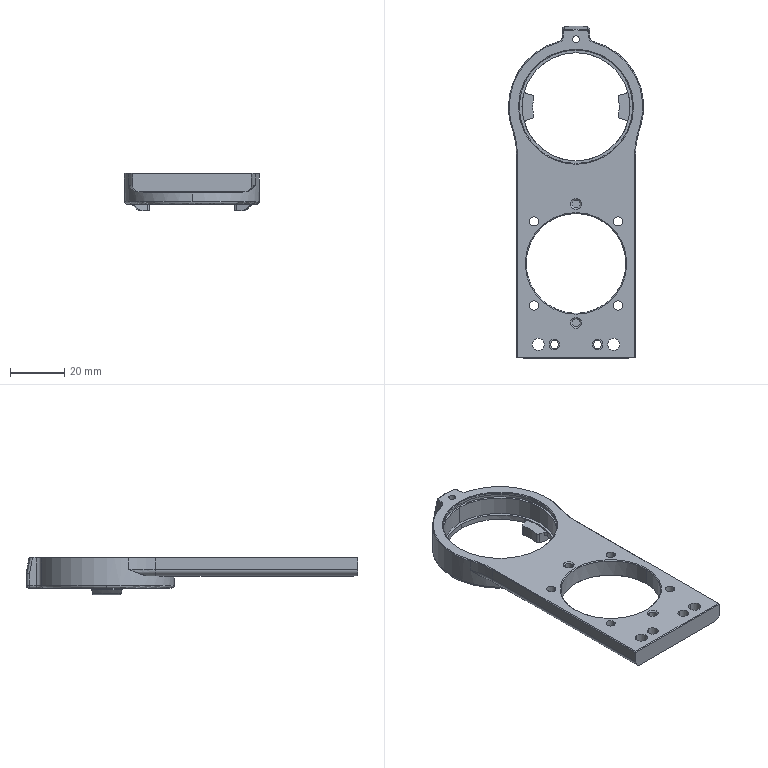NC program | NX | posted with a generic post | part box 50 x 122.9 x 14 mm
Lines 19 to 852 of 4462:
(ZLEVEL_PROFILE , TOOL : D10)
N36 T15 M6
N38 G54
N40 G17 G0 G90 X-66.55 Y-13.852 S9500 M3
N42 G43 Z30. H15
N44 Z1.5
N46 G94 G1 Y22.554 Z-0.408 F1000.
N48 X-66.216 Y23.898 Z-0.481
N50 X-65.534 Y25.104 Z-0.553
N52 X-64.554 Y26.084 Z-0.626
N54 X-63.348 Y26.766 Z-0.698
N56 X-62.004 Y27.1 Z-0.771
N58 X-61.45 Z-0.8
N60 X13.634 F3500.
N62 G3 X21.745 Y28.458 R24.9
N64 G2 X59.92 Y10.056 R30.1
N66 X65.193 Y4.632 R6.157
N68 X65.162 Y-4.852 R34.086
N70 X59.926 Y-10.04 R6.113
N72 X21.745 Y-28.458 R30.1
N74 G3 X13.634 Y-27.1 R24.9
N76 G1 X-61.45
N78 G2 X-66.55 Y-22. R5.1
N80 G1 Y22.
N82 G2 X-61.45 Y27.1 R5.1
N84 G1 X13.634 Z-0.973
N86 X14.666 Y27.121 Z-0.976
N88 X15.697 Y27.186 Z-0.978
N90 X16.724 Y27.293 Z-0.981
N92 X17.746 Y27.442 Z-0.983
N94 X18.76 Y27.634 Z-0.985
N96 X19.766 Y27.867 Z-0.988
N98 X20.762 Y28.142 Z-0.99
N100 X21.745 Y28.458 Z-0.992
N102 X22.988 Y28.857 Z-0.996
N104 X24.248 Y29.201 Z-0.999
N106 X25.522 Y29.49 Z-1.002
N108 X26.806 Y29.724 Z-1.005
N110 X28.1 Y29.902 Z-1.008
N112 X29.4 Y30.023 Z-1.011
N114 X30.704 Y30.088 Z-1.014
N116 X32.01 Y30.096 Z-1.017
N118 X33.315 Y30.048 Z-1.02
N120 X34.617 Y29.943 Z-1.023
N122 X35.913 Y29.782 Z-1.026
N124 X37.2 Y29.565 Z-1.029
N126 X38.478 Y29.292 Z-1.032
N128 X39.742 Y28.964 Z-1.035
N130 X40.99 Y28.581 Z-1.038
N132 X42.221 Y28.145 Z-1.041
N134 X43.432 Y27.656 Z-1.044
N136 X44.62 Y27.114 Z-1.047
N138 X45.784 Y26.522 Z-1.05
N140 X46.921 Y25.88 Z-1.053
N142 X48.029 Y25.188 Z-1.056
N144 X49.106 Y24.45 Z-1.059
N146 X50.15 Y23.666 Z-1.062
N148 X51.159 Y22.837 Z-1.065
N150 X52.131 Y21.965 Z-1.068
N152 X53.064 Y21.051 Z-1.071
N154 X53.957 Y20.098 Z-1.074
N156 X54.808 Y19.107 Z-1.077
N158 X55.615 Y18.081 Z-1.08
N160 X56.376 Y17.02 Z-1.083
N162 X57.091 Y15.927 Z-1.086
N164 X57.758 Y14.804 Z-1.089
N166 X58.375 Y13.654 Z-1.092
N168 X58.942 Y12.477 Z-1.095
N170 X59.452 Y11.291 Z-1.098
N172 X59.923 Y10.052 Z-1.101
N174 X60.494 Y9.952 Z-1.102
N176 X61.054 Y9.797 Z-1.104
N178 X61.6 Y9.593 Z-1.105
N180 X62.124 Y9.337 Z-1.106
N182 X62.376 Y9.189 Z-1.107
N184 X62.622 Y9.031 Z-1.108
N186 X62.859 Y8.861
N188 X63.085 Y8.674 Z-1.109
N190 X63.519 Y8.28 Z-1.11
N192 X63.913 Y7.846 Z-1.112
N194 X64.261 Y7.374 Z-1.113
N196 X64.566 Y6.872 Z-1.115
N198 X64.816 Y6.341 Z-1.116
N200 X65.015 Y5.787 Z-1.117
N202 X65.141 Y5.317 Z-1.118
N204 X65.23 Y4.838 Z-1.119
N206 X65.256 Y4.64 Z-1.12
N208 X65.393 Y3.457 Z-1.123
N210 X65.499 Y2.27 Z-1.125
N212 X65.558 Y1.08 Z-1.128
N214 X65.577 Y-0.111 Z-1.131
N216 X65.549 Y-1.303 Z-1.134
N218 X65.486 Y-2.492 Z-1.136
N220 X65.373 Y-3.679 Z-1.139
N222 X65.231 Y-4.862 Z-1.142
N224 X65.121 Y-5.423 Z-1.143
N226 X64.961 Y-5.971 Z-1.145
N228 X64.752 Y-6.503 Z-1.146
N230 X64.494 Y-7.012 Z-1.147
N232 X64.188 Y-7.493 Z-1.149
N234 X63.839 Y-7.945 Z-1.15
N236 X63.448 Y-8.36 Z-1.151
N238 X63.025 Y-8.74 Z-1.152
N240 X62.563 Y-9.073 Z-1.154
N242 X62.076 Y-9.366 Z-1.155
N244 X61.565 Y-9.614 Z-1.156
N246 X61.032 Y-9.807 Z-1.158
N248 X60.485 Y-9.957 Z-1.159
N250 X59.927 Y-10.05 Z-1.16
N252 X59.456 Y-11.281 Z-1.163
N254 X58.949 Y-12.463 Z-1.166
N256 X58.382 Y-13.64 Z-1.169
N258 X57.765 Y-14.791 Z-1.172
N260 X57.099 Y-15.915 Z-1.175
N262 X56.384 Y-17.008 Z-1.178
N264 X55.623 Y-18.07 Z-1.181
N266 X54.816 Y-19.097 Z-1.184
N268 X53.965 Y-20.089 Z-1.187
N270 X53.073 Y-21.042 Z-1.191
N272 X52.139 Y-21.956 Z-1.194
N274 X51.167 Y-22.829 Z-1.197
N276 X50.158 Y-23.659 Z-1.2
N278 X49.114 Y-24.444 Z-1.203
N280 X48.037 Y-25.183 Z-1.206
N282 X46.929 Y-25.875 Z-1.209
N284 X45.792 Y-26.518 Z-1.212
N286 X44.628 Y-27.111 Z-1.215
N288 X43.439 Y-27.653 Z-1.218
N290 X42.228 Y-28.142 Z-1.221
N292 X40.997 Y-28.579 Z-1.224
N294 X39.748 Y-28.962 Z-1.227
N296 X38.483 Y-29.291 Z-1.23
N298 X37.206 Y-29.564 Z-1.233
N300 X35.918 Y-29.781 Z-1.236
N302 X34.622 Y-29.943 Z-1.239
N304 X33.32 Y-30.048 Z-1.242
N306 X32.014 Y-30.096 Z-1.245
N308 X30.708 Y-30.088 Z-1.248
N310 X29.403 Y-30.023 Z-1.251
N312 X28.102 Y-29.902 Z-1.254
N314 X26.808 Y-29.724 Z-1.257
N316 X25.523 Y-29.49 Z-1.26
N318 X24.249 Y-29.201 Z-1.263
N320 X22.989 Y-28.857 Z-1.266
N322 X21.745 Y-28.458 Z-1.269
N324 X20.762 Y-28.142 Z-1.271
N326 X19.766 Y-27.867 Z-1.274
N328 X18.76 Y-27.634 Z-1.276
N330 X17.746 Y-27.442 Z-1.278
N332 X16.724 Y-27.293 Z-1.281
N334 X15.697 Y-27.186 Z-1.283
N336 X14.666 Y-27.121 Z-1.286
N338 X13.634 Y-27.1 Z-1.288
N340 X-61.45 Z-1.461
N342 X-61.95 Y-27.075 Z-1.463
N344 X-62.445 Y-27.002 Z-1.464
N346 X-62.93 Y-26.88 Z-1.465
N348 X-63.402 Y-26.712 Z-1.466
N350 X-63.854 Y-26.498 Z-1.467
N352 X-64.283 Y-26.24 Z-1.468
N354 X-64.685 Y-25.942 Z-1.47
N356 X-65.056 Y-25.606 Z-1.471
N358 X-65.392 Y-25.235 Z-1.472
N360 X-65.69 Y-24.833 Z-1.473
N362 X-65.948 Y-24.404 Z-1.474
N364 X-66.162 Y-23.952 Z-1.475
N366 X-66.33 Y-23.48 Z-1.476
N368 X-66.452 Y-22.995 Z-1.478
N370 X-66.525 Y-22.5 Z-1.479
N372 X-66.55 Y-22. Z-1.48
N374 Y22. Z-1.582
N376 X-66.525 Y22.5 Z-1.583
N378 X-66.452 Y22.995 Z-1.584
N380 X-66.33 Y23.48 Z-1.585
N382 X-66.162 Y23.952 Z-1.586
N384 X-65.948 Y24.404 Z-1.587
N386 X-65.69 Y24.833 Z-1.588
N388 X-65.392 Y25.235 Z-1.59
N390 X-65.056 Y25.606 Z-1.591
N392 X-64.685 Y25.942 Z-1.592
N394 X-64.283 Y26.24 Z-1.593
N396 X-63.854 Y26.498 Z-1.594
N398 X-63.402 Y26.712 Z-1.595
N400 X-62.93 Y26.88 Z-1.597
N402 X-62.445 Y27.002 Z-1.598
N404 X-61.95 Y27.075 Z-1.599
N406 X-61.45 Y27.1 Z-1.6
N408 X13.634 Z-1.773
N410 X14.666 Y27.121 Z-1.776
N412 X15.697 Y27.186 Z-1.778
N414 X16.724 Y27.293 Z-1.78
N416 X17.746 Y27.442 Z-1.783
N418 X18.76 Y27.634 Z-1.785
N420 X19.766 Y27.867 Z-1.788
N422 X20.762 Y28.142 Z-1.79
N424 X21.745 Y28.458 Z-1.792
N426 X22.988 Y28.857 Z-1.795
N428 X24.248 Y29.201 Z-1.798
N430 X25.522 Y29.49 Z-1.801
N432 X26.806 Y29.724 Z-1.804
N434 X28.1 Y29.902 Z-1.807
N436 X29.4 Y30.023 Z-1.81
N438 X30.704 Y30.088 Z-1.813
N440 X32.01 Y30.096 Z-1.816
N442 X33.315 Y30.048 Z-1.819
N444 X34.617 Y29.943 Z-1.822
N446 X35.913 Y29.782 Z-1.825
N448 X37.2 Y29.565 Z-1.828
N450 X38.478 Y29.292 Z-1.831
N452 X39.742 Y28.964 Z-1.835
N454 X40.99 Y28.581 Z-1.838
N456 X42.221 Y28.145 Z-1.841
N458 X43.432 Y27.656 Z-1.844
N460 X44.62 Y27.114 Z-1.847
N462 X45.784 Y26.522 Z-1.85
N464 X46.921 Y25.88 Z-1.853
N466 X48.029 Y25.188 Z-1.856
N468 X49.106 Y24.45 Z-1.859
N470 X50.15 Y23.666 Z-1.862
N472 X51.159 Y22.837 Z-1.865
N474 X52.131 Y21.965 Z-1.868
N476 X53.064 Y21.051 Z-1.871
N478 X53.957 Y20.098 Z-1.874
N480 X54.808 Y19.107 Z-1.877
N482 X55.615 Y18.081 Z-1.88
N484 X56.376 Y17.02 Z-1.883
N486 X57.091 Y15.927 Z-1.886
N488 X57.758 Y14.804 Z-1.889
N490 X58.375 Y13.654 Z-1.892
N492 X58.942 Y12.477 Z-1.895
N494 X59.449 Y11.298 Z-1.898
N496 X59.921 Y10.068 Z-1.901
N498 X60.492 Y9.979 Z-1.902
N500 X61.054 Y9.844 Z-1.903
N502 X61.601 Y9.655 Z-1.905
N504 X62.128 Y9.415 Z-1.906
N506 X62.385 Y9.28 Z-1.907
N508 X62.631 Y9.128
N510 X62.871 Y8.964 Z-1.908
N512 X63.102 Y8.788 Z-1.909
N514 X63.545 Y8.413 Z-1.91
N516 X63.948 Y7.994 Z-1.911
N518 X64.309 Y7.538 Z-1.913
N520 X64.626 Y7.05 Z-1.914
N522 X64.893 Y6.532 Z-1.915
N524 X65.108 Y5.991 Z-1.917
N526 X65.274 Y5.432 Z-1.918
N528 X65.387 Y4.86 Z-1.92
N530 X65.532 Y3.65 Z-1.922
N532 X65.648 Y2.436 Z-1.925
N534 X65.712 Y1.219 Z-1.928
N536 X65.738 Y0. Z-1.931
N538 X65.713 Y-1.219 Z-1.934
N540 X65.65 Y-2.436 Z-1.936
N542 X65.536 Y-3.65 Z-1.939
N544 X65.392 Y-4.861 Z-1.942
N546 X65.279 Y-5.433 Z-1.943
N548 X65.113 Y-5.992 Z-1.945
N550 X64.898 Y-6.534 Z-1.946
N552 X64.631 Y-7.053 Z-1.947
N554 X64.314 Y-7.542 Z-1.949
N556 X63.952 Y-7.998 Z-1.95
N558 X63.549 Y-8.418 Z-1.951
N560 X63.107 Y-8.796 Z-1.953
N562 X62.635 Y-9.134 Z-1.954
N564 X62.131 Y-9.422 Z-1.955
N566 X61.602 Y-9.659 Z-1.957
N568 X61.054 Y-9.848 Z-1.958
N570 X60.491 Y-9.981 Z-1.959
N572 X59.921 Y-10.069 Z-1.961
N574 X59.449 Y-11.299 Z-1.964
N576 X58.941 Y-12.479 Z-1.967
N578 X58.374 Y-13.655 Z-1.97
N580 X57.757 Y-14.806 Z-1.973
N582 X57.09 Y-15.929 Z-1.976
N584 X56.375 Y-17.021 Z-1.979
N586 X55.613 Y-18.082 Z-1.982
N588 X54.807 Y-19.109 Z-1.985
N590 X53.956 Y-20.099 Z-1.988
N592 X53.063 Y-21.052 Z-1.991
N594 X52.13 Y-21.966 Z-1.994
N596 X51.158 Y-22.838 Z-1.997
N598 X50.149 Y-23.666 Z-2.
N600 X49.105 Y-24.451 Z-2.003
N602 X48.028 Y-25.189 Z-2.006
N604 X46.92 Y-25.88 Z-2.009
N606 X45.783 Y-26.522 Z-2.012
N608 X44.619 Y-27.115 Z-2.015
N610 X43.431 Y-27.656 Z-2.018
N612 X42.22 Y-28.145 Z-2.021
N614 X40.989 Y-28.582 Z-2.024
N616 X39.741 Y-28.964 Z-2.027
N618 X38.477 Y-29.292 Z-2.03
N620 X37.2 Y-29.565 Z-2.033
N622 X35.912 Y-29.782 Z-2.036
N624 X34.616 Y-29.943 Z-2.039
N626 X33.315 Y-30.048 Z-2.042
N628 X32.01 Y-30.096 Z-2.045
N630 X30.704 Y-30.088 Z-2.048
N632 X29.4 Y-30.023 Z-2.051
N634 X28.1 Y-29.902 Z-2.054
N636 X26.806 Y-29.724 Z-2.057
N638 X25.521 Y-29.49 Z-2.06
N640 X24.248 Y-29.201 Z-2.063
N642 X22.988 Y-28.857 Z-2.066
N644 X21.745 Y-28.458 Z-2.069
N646 X20.762 Y-28.142 Z-2.072
N648 X19.766 Y-27.867 Z-2.074
N650 X18.76 Y-27.634 Z-2.076
N652 X17.746 Y-27.442 Z-2.079
N654 X16.724 Y-27.293 Z-2.081
N656 X15.697 Y-27.186 Z-2.084
N658 X14.666 Y-27.121 Z-2.086
N660 X13.634 Y-27.1 Z-2.088
N662 X-61.45 Z-2.262
N664 X-61.95 Y-27.075 Z-2.263
N666 X-62.445 Y-27.002 Z-2.264
N668 X-62.93 Y-26.88 Z-2.265
N670 X-63.402 Y-26.712 Z-2.266
N672 X-63.854 Y-26.498 Z-2.267
N674 X-64.283 Y-26.24 Z-2.268
N676 X-64.685 Y-25.942 Z-2.27
N678 X-65.056 Y-25.606 Z-2.271
N680 X-65.392 Y-25.235 Z-2.272
N682 X-65.69 Y-24.833 Z-2.273
N684 X-65.948 Y-24.404 Z-2.274
N686 X-66.162 Y-23.952 Z-2.275
N688 X-66.33 Y-23.48 Z-2.277
N690 X-66.452 Y-22.995 Z-2.278
N692 X-66.525 Y-22.5 Z-2.279
N694 X-66.55 Y-22. Z-2.28
N696 Y22. Z-2.382
N698 X-66.525 Y22.5 Z-2.383
N700 X-66.452 Y22.995 Z-2.384
N702 X-66.33 Y23.48 Z-2.385
N704 X-66.162 Y23.952 Z-2.386
N706 X-65.948 Y24.404 Z-2.387
N708 X-65.69 Y24.833 Z-2.388
N710 X-65.392 Y25.235 Z-2.39
N712 X-65.056 Y25.606 Z-2.391
N714 X-64.685 Y25.942 Z-2.392
N716 X-64.283 Y26.24 Z-2.393
N718 X-63.854 Y26.498 Z-2.394
N720 X-63.402 Y26.712 Z-2.395
N722 X-62.93 Y26.88 Z-2.397
N724 X-62.445 Y27.002 Z-2.398
N726 X-61.95 Y27.075 Z-2.399
N728 X-61.45 Y27.1 Z-2.4
N730 X13.634 Z-2.508
N732 X14.666 Y27.121 Z-2.51
N734 X15.697 Y27.186 Z-2.511
N736 X16.724 Y27.293 Z-2.513
N738 X17.746 Y27.442 Z-2.514
N740 X18.76 Y27.634 Z-2.516
N742 X19.766 Y27.867 Z-2.517
N744 X20.762 Y28.142 Z-2.519
N746 X21.745 Y28.458 Z-2.52
N748 X22.988 Y28.857 Z-2.522
N750 X24.247 Y29.201 Z-2.524
N752 X25.52 Y29.49 Z-2.526
N754 X26.805 Y29.724 Z-2.528
N756 X28.098 Y29.901 Z-2.53
N758 X29.398 Y30.023 Z-2.531
N760 X30.702 Y30.088 Z-2.533
N762 X32.007 Y30.097 Z-2.535
N764 X33.312 Y30.048 Z-2.537
N766 X34.613 Y29.944 Z-2.539
N768 X35.909 Y29.783 Z-2.541
N770 X37.196 Y29.566 Z-2.543
N772 X38.473 Y29.293 Z-2.545
N774 X39.736 Y28.965 Z-2.546
N776 X40.985 Y28.583 Z-2.548
N778 X42.215 Y28.147 Z-2.55
N780 X43.426 Y27.658 Z-2.552
N782 X44.614 Y27.117 Z-2.554
N784 X45.778 Y26.525 Z-2.556
N786 X46.914 Y25.883 Z-2.558
N788 X48.022 Y25.193 Z-2.56
N790 X49.099 Y24.455 Z-2.562
N792 X50.143 Y23.671 Z-2.563
N794 X51.152 Y22.842 Z-2.565
N796 X52.124 Y21.971 Z-2.567
N798 X53.057 Y21.058 Z-2.569
N800 X53.95 Y20.106 Z-2.571
N802 X54.801 Y19.115 Z-2.573
N804 X55.608 Y18.089 Z-2.575
N806 X56.37 Y17.029 Z-2.577
N808 X57.085 Y15.937 Z-2.578
N810 X57.752 Y14.815 Z-2.58
N812 X58.37 Y13.665 Z-2.582
N814 X58.937 Y12.489 Z-2.584
N816 X59.446 Y11.307 Z-2.586
N818 X59.916 Y10.069 Z-2.588
N820 X60.501 Y9.997 Z-2.589
N822 X61.078 Y9.879 Z-2.59
N824 X61.637 Y9.69
N826 X62.181 Y9.462 Z-2.591
N828 X62.444 Y9.326 Z-2.592
N830 X62.698 Y9.176
N832 X62.943 Y9.011 Z-2.593
N834 X63.18 Y8.834
N836 X63.415 Y8.653
N838 X63.636 Y8.458 Z-2.594
N840 X63.847 Y8.25
N842 X64.05 Y8.035 Z-2.595
N844 X64.419 Y7.572
N846 X64.746 Y7.079 Z-2.596
N848 X65.02 Y6.554 Z-2.597
N850 X65.239 Y6.003 Z-2.598
N852 X65.41 Y5.436 Z-2.599
N854 X65.525 Y4.855 Z-2.6
N856 X65.556 Y4.624
N858 X65.685 Y3.53 Z-2.602
N860 X65.784 Y2.434 Z-2.603
N862 X65.848 Y1.219 Z-2.605
N864 X65.873 Y0.002 Z-2.607
N866 X65.849 Y-1.215 Z-2.609
N868 X65.786 Y-2.431 Z-2.61
N870 X65.687 Y-3.529 Z-2.612
N872 X65.559 Y-4.624 Z-2.613
N874 X65.529 Y-4.851 Z-2.614
N876 X65.413 Y-5.433 Z-2.615
N878 X65.243 Y-6.001
N880 X65.139 Y-6.28 Z-2.616
N882 X65.024 Y-6.553
N884 X64.894 Y-6.819 Z-2.617
N886 X64.75 Y-7.079
N888 X64.425 Y-7.574 Z-2.618
N890 X64.053 Y-8.036 Z-2.619
N892 X63.639 Y-8.46 Z-2.62
N894 X63.418 Y-8.656
N896 X63.183 Y-8.837 Z-2.621
N898 X62.945 Y-9.014
N900 X62.7 Y-9.179
N902 X62.445 Y-9.329 Z-2.622
N904 X62.182 Y-9.464
N906 X61.637 Y-9.693 Z-2.623
N908 X61.078 Y-9.881 Z-2.624
N910 X60.499 Y-9.998 Z-2.625
N912 X59.915 Y-10.079 Z-2.626
N914 X59.444 Y-11.311 Z-2.628
N916 X58.936 Y-12.491 Z-2.629
N918 X58.368 Y-13.667 Z-2.631
N920 X57.751 Y-14.817 Z-2.633
N922 X57.084 Y-15.939 Z-2.635
N924 X56.368 Y-17.031 Z-2.637
N926 X55.607 Y-18.091 Z-2.639
N928 X54.8 Y-19.117 Z-2.641
N930 X53.949 Y-20.107 Z-2.643
N932 X53.056 Y-21.06 Z-2.645
N934 X52.123 Y-21.972 Z-2.646
N936 X51.151 Y-22.844 Z-2.648
N938 X50.142 Y-23.672 Z-2.65
N940 X49.098 Y-24.456 Z-2.652
N942 X48.021 Y-25.194 Z-2.654
N944 X46.913 Y-25.884 Z-2.656
N946 X45.776 Y-26.526 Z-2.658
N948 X44.613 Y-27.118 Z-2.66
N950 X43.425 Y-27.659 Z-2.661
N952 X42.214 Y-28.148 Z-2.663
N954 X40.984 Y-28.583 Z-2.665
N956 X39.735 Y-28.966 Z-2.667
N958 X38.472 Y-29.293 Z-2.669
N960 X37.195 Y-29.566 Z-2.671
N962 X35.908 Y-29.783 Z-2.673
N964 X34.612 Y-29.944 Z-2.675
N966 X33.311 Y-30.048 Z-2.676
N968 X32.007 Y-30.097 Z-2.678
N970 X30.701 Y-30.088 Z-2.68
N972 X29.398 Y-30.023 Z-2.682
N974 X28.098 Y-29.901 Z-2.684
N976 X26.805 Y-29.724 Z-2.686
N978 X25.52 Y-29.49 Z-2.688
N980 X24.247 Y-29.201 Z-2.69
N982 X22.988 Y-28.857 Z-2.692
N984 X21.745 Y-28.458 Z-2.693
N986 X20.762 Y-28.142 Z-2.695
N988 X19.766 Y-27.867 Z-2.696
N990 X18.76 Y-27.634 Z-2.698
N992 X17.746 Y-27.442 Z-2.699
N994 X16.724 Y-27.293 Z-2.701
N996 X15.697 Y-27.186 Z-2.702
N998 X14.666 Y-27.121 Z-2.704
N1000 X13.634 Y-27.1 Z-2.705
N1002 X-61.45 Z-2.814
N1004 X-61.95 Y-27.075
N1006 X-62.445 Y-27.002 Z-2.815
N1008 X-62.93 Y-26.88 Z-2.816
N1010 X-63.402 Y-26.712
N1012 X-63.854 Y-26.498 Z-2.817
N1014 X-64.283 Y-26.24 Z-2.818
N1016 X-64.685 Y-25.942 Z-2.819
N1018 X-65.056 Y-25.606
N1020 X-65.392 Y-25.235 Z-2.82
N1022 X-65.69 Y-24.833 Z-2.821
N1024 X-65.948 Y-24.404
N1026 X-66.162 Y-23.952 Z-2.822
N1028 X-66.33 Y-23.48 Z-2.823
N1030 X-66.452 Y-22.995 Z-2.824
N1032 X-66.525 Y-22.5
N1034 X-66.55 Y-22. Z-2.825
N1036 Y22. Z-2.888
N1038 X-66.525 Y22.5 Z-2.889
N1040 X-66.452 Y22.995 Z-2.89
N1042 X-66.33 Y23.48 Z-2.891
N1044 X-66.162 Y23.952
N1046 X-65.948 Y24.404 Z-2.892
N1048 X-65.69 Y24.833 Z-2.893
N1050 X-65.392 Y25.235 Z-2.894
N1052 X-65.056 Y25.606
N1054 X-64.685 Y25.942 Z-2.895
N1056 X-64.283 Y26.24 Z-2.896
N1058 X-63.854 Y26.498
N1060 X-63.402 Y26.712 Z-2.897
N1062 X-62.93 Y26.88 Z-2.898
N1064 X-62.445 Y27.002 Z-2.899
N1066 X-61.95 Y27.075
N1068 X-61.45 Y27.1 Z-2.9
N1070 X13.634 Z-3.116
N1072 X14.666 Y27.121 Z-3.119
N1074 X15.697 Y27.186 Z-3.122
N1076 X16.724 Y27.293 Z-3.125
N1078 X17.746 Y27.442 Z-3.128
N1080 X18.76 Y27.634 Z-3.131
N1082 X19.766 Y27.867 Z-3.134
N1084 X20.762 Y28.142 Z-3.137
N1086 X21.745 Y28.458 Z-3.14
N1088 X22.988 Y28.856 Z-3.144
N1090 X24.247 Y29.201 Z-3.148
N1092 X25.519 Y29.49 Z-3.151
N1094 X26.803 Y29.723 Z-3.155
N1096 X28.096 Y29.901 Z-3.159
N1098 X29.396 Y30.023 Z-3.163
N1100 X30.699 Y30.088 Z-3.166
N1102 X32.004 Y30.097 Z-3.17
N1104 X33.308 Y30.049 Z-3.174
N1106 X34.609 Y29.944 Z-3.178
N1108 X35.905 Y29.783 Z-3.181
N1110 X37.192 Y29.567 Z-3.185
N1112 X38.468 Y29.294 Z-3.189
N1114 X39.731 Y28.967 Z-3.193
N1116 X40.979 Y28.585 Z-3.196
N1118 X42.21 Y28.149 Z-3.2
N1120 X43.42 Y27.661 Z-3.204
N1122 X44.608 Y27.12 Z-3.208
N1124 X45.771 Y26.529 Z-3.211
N1126 X46.908 Y25.887 Z-3.215
N1128 X48.015 Y25.197 Z-3.219
N1130 X49.092 Y24.46 Z-3.223
N1132 X50.136 Y23.676 Z-3.226
N1134 X51.145 Y22.848 Z-3.23
N1136 X52.117 Y21.977 Z-3.234
N1138 X53.05 Y21.065 Z-3.238
N1140 X53.943 Y20.113 Z-3.242
N1142 X54.794 Y19.124 Z-3.245
N1144 X55.601 Y18.098 Z-3.249
N1146 X56.363 Y17.039 Z-3.253
N1148 X57.079 Y15.947 Z-3.257
N1150 X57.746 Y14.825 Z-3.26
N1152 X58.364 Y13.676 Z-3.264
N1154 X58.931 Y12.501 Z-3.268
N1156 X59.44 Y11.32 Z-3.272
N1158 X59.911 Y10.082 Z-3.275
N1160 X60.444 Y10.025 Z-3.277
N1162 X60.974 Y9.941 Z-3.278
N1164 X61.489 Y9.789 Z-3.28
N1166 X61.996 Y9.61 Z-3.282
N1168 X62.482 Y9.378 Z-3.283
N1170 X62.947 Y9.106 Z-3.285
N1172 X63.386 Y8.791 Z-3.286
N1174 X63.794 Y8.437 Z-3.288
N1176 X64.173 Y8.052 Z-3.289
N1178 X64.515 Y7.633 Z-3.291
N1180 X64.82 Y7.185 Z-3.292
N1182 X65.086 Y6.713 Z-3.294
N1184 X65.301 Y6.215 Z-3.296
N1186 X65.478 Y5.703 Z-3.297
N1188 X65.61 Y5.176 Z-3.299
N1190 X65.696 Y4.641 Z-3.3
N1192 X65.831 Y3.485 Z-3.304
N1194 X65.933 Y2.327 Z-3.307
N1196 X65.991 Y1.164 Z-3.31
N1198 X66.014 Y0. Z-3.314
N1200 X65.992 Y-1.164 Z-3.317
N1202 X65.935 Y-2.327 Z-3.32
N1204 X65.835 Y-3.486 Z-3.324
N1206 X65.701 Y-4.641 Z-3.327
N1208 X65.615 Y-5.177 Z-3.329
N1210 X65.484 Y-5.704 Z-3.33
N1212 X65.306 Y-6.217 Z-3.332
N1214 X65.093 Y-6.716 Z-3.333
N1216 X64.826 Y-7.188 Z-3.335
N1218 X64.524 Y-7.639 Z-3.336
N1220 X64.179 Y-8.056 Z-3.338
N1222 X63.802 Y-8.445 Z-3.339
N1224 X63.385 Y-8.789 Z-3.341
N1226 X62.952 Y-9.111 Z-3.343
N1228 X62.478 Y-9.367 Z-3.344
N1230 X61.998 Y-9.611 Z-3.346
N1232 X61.491 Y-9.792 Z-3.347
N1234 X60.975 Y-9.944 Z-3.349
N1236 X60.445 Y-10.026 Z-3.35
N1238 X59.912 Y-10.09 Z-3.352
N1240 X59.44 Y-11.321 Z-3.356
N1242 X58.932 Y-12.498 Z-3.359
N1244 X58.365 Y-13.674 Z-3.363
N1246 X57.747 Y-14.823 Z-3.367
N1248 X57.08 Y-15.945 Z-3.371
N1250 X56.364 Y-17.037 Z-3.374
N1252 X55.603 Y-18.097 Z-3.378
N1254 X54.795 Y-19.122 Z-3.382
N1256 X53.945 Y-20.112 Z-3.386
N1258 X53.052 Y-21.064 Z-3.389
N1260 X52.118 Y-21.976 Z-3.393
N1262 X51.146 Y-22.847 Z-3.397
N1264 X50.137 Y-23.675 Z-3.401
N1266 X49.094 Y-24.459 Z-3.404
N1268 X48.017 Y-25.196 Z-3.408
N1270 X46.909 Y-25.887 Z-3.412
N1272 X45.772 Y-26.528 Z-3.416
N1274 X44.609 Y-27.12 Z-3.42
N1276 X43.421 Y-27.66 Z-3.423
N1278 X42.211 Y-28.149 Z-3.427
N1280 X40.98 Y-28.585 Z-3.431
N1282 X39.732 Y-28.967 Z-3.435
N1284 X38.469 Y-29.294 Z-3.438
N1286 X37.192 Y-29.566 Z-3.442
N1288 X35.905 Y-29.783 Z-3.446
N1290 X34.61 Y-29.944 Z-3.45
N1292 X33.309 Y-30.049 Z-3.453
N1294 X32.005 Y-30.097 Z-3.457
N1296 X30.7 Y-30.088 Z-3.461
N1298 X29.396 Y-30.023 Z-3.465
N1300 X28.097 Y-29.901 Z-3.468
N1302 X26.804 Y-29.723 Z-3.472
N1304 X25.519 Y-29.49 Z-3.476
N1306 X24.247 Y-29.201 Z-3.48
N1308 X22.988 Y-28.856 Z-3.483
N1310 X21.745 Y-28.458 Z-3.487
N1312 X20.762 Y-28.142 Z-3.49
N1314 X19.766 Y-27.867 Z-3.493
N1316 X18.76 Y-27.634 Z-3.496
N1318 X17.746 Y-27.442 Z-3.499
N1320 X16.724 Y-27.293 Z-3.502
N1322 X15.697 Y-27.186 Z-3.505
N1324 X14.666 Y-27.121 Z-3.508
N1326 X13.634 Y-27.1 Z-3.511
N1328 X-61.45 Z-3.727
N1330 X-61.95 Y-27.075 Z-3.729
N1332 X-62.445 Y-27.002 Z-3.73
N1334 X-62.93 Y-26.88 Z-3.732
N1336 X-63.402 Y-26.712 Z-3.733
N1338 X-63.854 Y-26.498 Z-3.734
N1340 X-64.283 Y-26.24 Z-3.736
N1342 X-64.685 Y-25.942 Z-3.737
N1344 X-65.056 Y-25.606 Z-3.739
N1346 X-65.392 Y-25.235 Z-3.74
N1348 X-65.69 Y-24.833 Z-3.742
N1350 X-65.948 Y-24.404 Z-3.743
N1352 X-66.162 Y-23.952 Z-3.744
N1354 X-66.33 Y-23.48 Z-3.746
N1356 X-66.452 Y-22.995 Z-3.747
N1358 X-66.525 Y-22.5 Z-3.749
N1360 X-66.55 Y-22. Z-3.75
N1362 Y22. Z-3.877
N1364 X-66.525 Y22.5 Z-3.878
N1366 X-66.452 Y22.995 Z-3.88
N1368 X-66.33 Y23.48 Z-3.881
N1370 X-66.162 Y23.952 Z-3.883
N1372 X-65.948 Y24.404 Z-3.884
N1374 X-65.69 Y24.833 Z-3.886
N1376 X-65.392 Y25.235 Z-3.887
N1378 X-65.056 Y25.606 Z-3.888
N1380 X-64.685 Y25.942 Z-3.89
N1382 X-64.283 Y26.24 Z-3.891
N1384 X-63.854 Y26.498 Z-3.893
N1386 X-63.402 Y26.712 Z-3.894
N1388 X-62.93 Y26.88 Z-3.896
N1390 X-62.445 Y27.002 Z-3.897
N1392 X-61.95 Y27.075 Z-3.899
N1394 X-61.45 Y27.1 Z-3.9
N1396 X13.634 Z-4.116
N1398 X14.666 Y27.121 Z-4.119
N1400 X15.697 Y27.186 Z-4.122
N1402 X16.724 Y27.293 Z-4.125
N1404 X17.746 Y27.442 Z-4.128
N1406 X18.76 Y27.634 Z-4.131
N1408 X19.766 Y27.867 Z-4.134
N1410 X20.762 Y28.142 Z-4.137
N1412 X21.745 Y28.458 Z-4.14
N1414 X22.987 Y28.856 Z-4.144
N1416 X24.246 Y29.2 Z-4.147
N1418 X25.518 Y29.489 Z-4.151
N1420 X26.802 Y29.723 Z-4.155
N1422 X28.094 Y29.901 Z-4.159
N1424 X29.393 Y30.023 Z-4.162
N1426 X30.696 Y30.088 Z-4.166
N1428 X32.001 Y30.097 Z-4.17
N1430 X33.305 Y30.049 Z-4.174
N1432 X34.605 Y29.945 Z-4.177
N1434 X35.9 Y29.784 Z-4.181
N1436 X37.187 Y29.567 Z-4.185
N1438 X38.463 Y29.295 Z-4.189
N1440 X39.726 Y28.968 Z-4.192
N1442 X40.974 Y28.587 Z-4.196
N1444 X42.203 Y28.152 Z-4.2
N1446 X43.413 Y27.663 Z-4.204
N1448 X44.601 Y27.123 Z-4.207
N1450 X45.764 Y26.532 Z-4.211
N1452 X46.901 Y25.891 Z-4.215
N1454 X48.008 Y25.202 Z-4.219
N1456 X49.085 Y24.465 Z-4.222
N1458 X50.129 Y23.682 Z-4.226
N1460 X51.138 Y22.855 Z-4.23
N1462 X52.11 Y21.984 Z-4.234
N1464 X53.043 Y21.073 Z-4.237
N1466 X53.936 Y20.122 Z-4.241
N1468 X54.787 Y19.133 Z-4.245
N1470 X55.594 Y18.108 Z-4.249
N1472 X56.356 Y17.049 Z-4.252
N1474 X57.072 Y15.958 Z-4.256
N1476 X57.739 Y14.837 Z-4.26
N1478 X58.358 Y13.688 Z-4.264
N1480 X58.926 Y12.513 Z-4.267
N1482 X59.435 Y11.334 Z-4.271
N1484 X59.906 Y10.096 Z-4.275
N1486 X60.453 Y10.049 Z-4.276
N1488 X60.998 Y9.982 Z-4.278
N1490 X61.529 Y9.839 Z-4.28
N1492 X62.053 Y9.672 Z-4.281
N1494 X62.55 Y9.432 Z-4.283
N1496 X63.039 Y9.177 Z-4.284
N1498 X63.494 Y8.863 Z-4.286
N1500 X63.918 Y8.508 Z-4.288
N1502 X64.314 Y8.121 Z-4.289
N1504 X64.67 Y7.696 Z-4.291
N1506 X64.987 Y7.241 Z-4.292
N1508 X65.263 Y6.76 Z-4.294
N1510 X65.49 Y6.253 Z-4.296
N1512 X65.674 Y5.728 Z-4.297
N1514 X65.808 Y5.189 Z-4.299
N1516 X65.898 Y4.641 Z-4.3
N1518 X66.033 Y3.485 Z-4.304
N1520 X66.133 Y2.327 Z-4.307
N1522 X66.19 Y1.164 Z-4.31
N1524 X66.214 Y0. Z-4.314
N1526 X66.192 Y-1.164 Z-4.317
N1528 X66.135 Y-2.327 Z-4.32
N1530 X66.037 Y-3.486 Z-4.324
N1532 X65.903 Y-4.641 Z-4.327
N1534 X65.815 Y-5.191 Z-4.329
N1536 X65.68 Y-5.73 Z-4.33
N1538 X65.494 Y-6.254 Z-4.332
N1540 X65.271 Y-6.764 Z-4.333
N1542 X64.993 Y-7.245 Z-4.335
N1544 X64.679 Y-7.703 Z-4.337
N1546 X64.319 Y-8.125 Z-4.338
N1548 X63.923 Y-8.513 Z-4.34
N1550 X63.494 Y-8.863 Z-4.341
N1552 X63.042 Y-9.182 Z-4.343
N1554 X62.553 Y-9.437 Z-4.345
N1556 X62.049 Y-9.66 Z-4.346
N1558 X61.529 Y-9.843 Z-4.348
N1560 X60.998 Y-9.984 Z-4.349
N1562 X60.453 Y-10.05 Z-4.351
N1564 X59.906 Y-10.1 Z-4.353
N1566 X59.434 Y-11.335 Z-4.356
N1568 X58.926 Y-12.513 Z-4.36
N1570 X58.358 Y-13.688 Z-4.364
N1572 X57.739 Y-14.837 Z-4.368
N1574 X57.072 Y-15.958 Z-4.371
N1576 X56.356 Y-17.049 Z-4.375
N1578 X55.594 Y-18.108 Z-4.379
N1580 X54.787 Y-19.133 Z-4.383
N1582 X53.936 Y-20.122 Z-4.386
N1584 X53.043 Y-21.073 Z-4.39
N1586 X52.11 Y-21.984 Z-4.394
N1588 X51.138 Y-22.855 Z-4.398
N1590 X50.129 Y-23.682 Z-4.401
N1592 X49.085 Y-24.465 Z-4.405
N1594 X48.008 Y-25.202 Z-4.409
N1596 X46.901 Y-25.891 Z-4.413
N1598 X45.764 Y-26.532 Z-4.416
N1600 X44.601 Y-27.123 Z-4.42
N1602 X43.413 Y-27.663 Z-4.424
N1604 X42.203 Y-28.152 Z-4.428
N1606 X40.974 Y-28.587 Z-4.431
N1608 X39.726 Y-28.968 Z-4.435
N1610 X38.463 Y-29.295 Z-4.439
N1612 X37.187 Y-29.567 Z-4.443
N1614 X35.9 Y-29.784 Z-4.446
N1616 X34.605 Y-29.945 Z-4.45
N1618 X33.305 Y-30.049 Z-4.454
N1620 X32.001 Y-30.097 Z-4.458
N1622 X30.696 Y-30.088 Z-4.461
N1624 X29.393 Y-30.023 Z-4.465
N1626 X28.094 Y-29.901 Z-4.469
N1628 X26.802 Y-29.723 Z-4.473
N1630 X25.518 Y-29.489 Z-4.476
N1632 X24.246 Y-29.2 Z-4.48
N1634 X22.987 Y-28.856 Z-4.484
N1636 X21.745 Y-28.458 Z-4.488
N1638 X20.762 Y-28.142 Z-4.491
N1640 X19.766 Y-27.867 Z-4.494
N1642 X18.76 Y-27.634 Z-4.497
N1644 X17.746 Y-27.442 Z-4.5
N1646 X16.724 Y-27.293 Z-4.502
N1648 X15.697 Y-27.186 Z-4.505
N1650 X14.666 Y-27.121 Z-4.508
N1652 X13.634 Y-27.1 Z-4.511
N1654 X-61.45 Z-4.727
N1656 X-61.95 Y-27.075 Z-4.729
N1658 X-62.445 Y-27.002 Z-4.73
N1660 X-62.93 Y-26.88 Z-4.732
N1662 X-63.402 Y-26.712 Z-4.733
N1664 X-63.854 Y-26.498 Z-4.735
N1666 X-64.283 Y-26.24 Z-4.736
N1668 X-64.685 Y-25.942 Z-4.737
N1670 X-65.056 Y-25.606 Z-4.739
N1672 X-65.392 Y-25.235 Z-4.74
N1674 X-65.69 Y-24.833 Z-4.742
N1676 X-65.948 Y-24.404 Z-4.743
N1678 X-66.162 Y-23.952 Z-4.745
N1680 X-66.33 Y-23.48 Z-4.746
N1682 X-66.452 Y-22.995 Z-4.748
N1684 X-66.525 Y-22.5 Z-4.749
N1686 X-66.55 Y-22. Z-4.75
N1688 Y22. Z-4.877
N1690 X-66.525 Y22.5 Z-4.878
N1692 X-66.452 Y22.995 Z-4.88
N1694 X-66.33 Y23.48 Z-4.881
N1696 X-66.162 Y23.952 Z-4.883